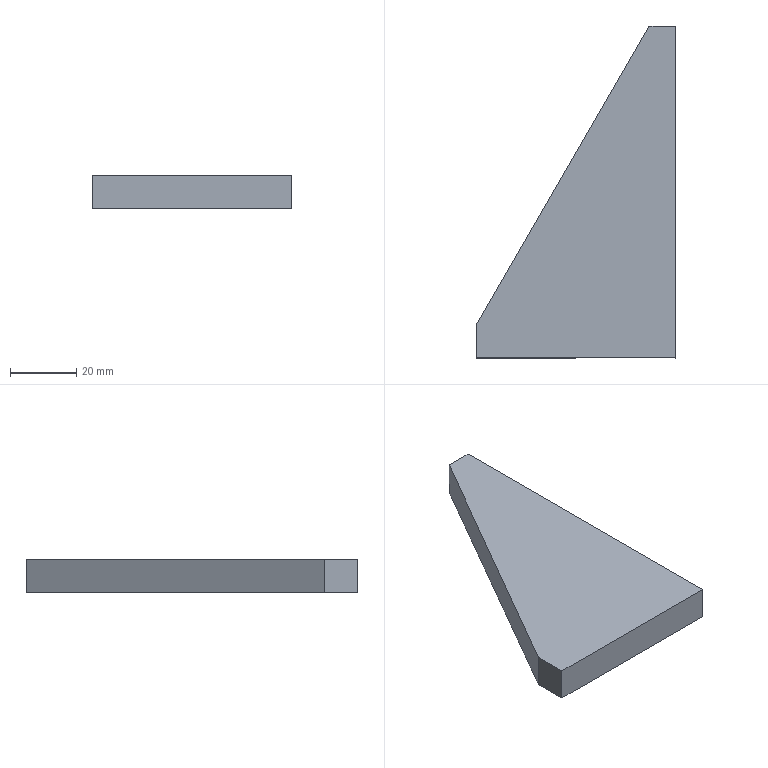Part | STEP file | X77-02104 | 1 solid | 7 faces | box 60 x 100 x 10 mm | volume 36617 mm3 | plane 7
STEP:
#1=CARTESIAN_POINT('',(-109.839,-76.534,0.));
#2=VERTEX_POINT('',#1);
#3=CARTESIAN_POINT('',(-109.839,23.466,0.));
#4=VERTEX_POINT('',#3);
#5=CARTESIAN_POINT('',(-109.839,23.466,0.));
#6=DIRECTION('',(0.,1.,0.));
#7=VECTOR('',#6,1000.);
#8=LINE('',#5,#7);
#9=EDGE_CURVE('',#2,#4,#8,.T.);
#10=ORIENTED_EDGE('',*,*,#9,.T.);
#11=CARTESIAN_POINT('',(-109.839,23.466,10.));
#12=VERTEX_POINT('',#11);
#13=CARTESIAN_POINT('',(-109.839,23.466,10.));
#14=DIRECTION('',(0.,0.,-1.));
#15=VECTOR('',#14,1000.);
#16=LINE('',#13,#15);
#17=EDGE_CURVE('',#12,#4,#16,.T.);
#18=ORIENTED_EDGE('',*,*,#17,.F.);
#19=CARTESIAN_POINT('',(-109.839,-76.534,10.));
#20=VERTEX_POINT('',#19);
#21=CARTESIAN_POINT('',(-109.839,23.466,10.));
#22=DIRECTION('',(0.,1.,0.));
#23=VECTOR('',#22,1000.);
#24=LINE('',#21,#23);
#25=EDGE_CURVE('',#20,#12,#24,.T.);
#26=ORIENTED_EDGE('',*,*,#25,.F.);
#27=CARTESIAN_POINT('',(-109.839,-76.534,10.));
#28=DIRECTION('',(0.,0.,-1.));
#29=VECTOR('',#28,1000.);
#30=LINE('',#27,#29);
#31=EDGE_CURVE('',#20,#2,#30,.T.);
#32=ORIENTED_EDGE('',*,*,#31,.T.);
#33=EDGE_LOOP('',(#10,#18,#26,#32));
#34=FACE_OUTER_BOUND('',#33,.T.);
#35=CARTESIAN_POINT('',(-109.839,23.466,10.));
#36=DIRECTION('',(-1.,0.,0.));
#37=DIRECTION('',(0.,-1.,0.));
#38=AXIS2_PLACEMENT_3D('',#35,#36,#37);
#39=PLANE('',#38);
#40=ADVANCED_FACE('',(#34),#39,.F.);
#41=CARTESIAN_POINT('',(-117.878,23.466,0.));
#42=VERTEX_POINT('',#41);
#43=CARTESIAN_POINT('',(-109.839,23.466,0.));
#44=DIRECTION('',(-1.,0.,0.));
#45=VECTOR('',#44,1000.);
#46=LINE('',#43,#45);
#47=EDGE_CURVE('',#4,#42,#46,.T.);
#48=ORIENTED_EDGE('',*,*,#47,.T.);
#49=CARTESIAN_POINT('',(-117.878,23.466,10.));
#50=VERTEX_POINT('',#49);
#51=CARTESIAN_POINT('',(-117.878,23.466,10.));
#52=DIRECTION('',(0.,0.,-1.));
#53=VECTOR('',#52,1000.);
#54=LINE('',#51,#53);
#55=EDGE_CURVE('',#50,#42,#54,.T.);
#56=ORIENTED_EDGE('',*,*,#55,.F.);
#57=CARTESIAN_POINT('',(-109.839,23.466,10.));
#58=DIRECTION('',(-1.,0.,0.));
#59=VECTOR('',#58,1000.);
#60=LINE('',#57,#59);
#61=EDGE_CURVE('',#12,#50,#60,.T.);
#62=ORIENTED_EDGE('',*,*,#61,.F.);
#63=ORIENTED_EDGE('',*,*,#17,.T.);
#64=EDGE_LOOP('',(#48,#56,#62,#63));
#65=FACE_OUTER_BOUND('',#64,.T.);
#66=CARTESIAN_POINT('',(-109.839,23.466,10.));
#67=DIRECTION('',(0.,-1.,0.));
#68=DIRECTION('',(0.,0.,-1.));
#69=AXIS2_PLACEMENT_3D('',#66,#67,#68);
#70=PLANE('',#69);
#71=ADVANCED_FACE('',(#65),#70,.F.);
#72=CARTESIAN_POINT('',(-169.839,-66.534,0.));
#73=VERTEX_POINT('',#72);
#74=CARTESIAN_POINT('',(-169.839,-66.534,0.));
#75=DIRECTION('',(-0.5,-0.866,0.));
#76=VECTOR('',#75,1000.);
#77=LINE('',#74,#76);
#78=EDGE_CURVE('',#42,#73,#77,.T.);
#79=ORIENTED_EDGE('',*,*,#78,.T.);
#80=CARTESIAN_POINT('',(-169.839,-66.534,10.));
#81=VERTEX_POINT('',#80);
#82=CARTESIAN_POINT('',(-169.839,-66.534,10.));
#83=DIRECTION('',(0.,0.,-1.));
#84=VECTOR('',#83,1000.);
#85=LINE('',#82,#84);
#86=EDGE_CURVE('',#81,#73,#85,.T.);
#87=ORIENTED_EDGE('',*,*,#86,.F.);
#88=CARTESIAN_POINT('',(-169.839,-66.534,10.));
#89=DIRECTION('',(-0.5,-0.866,0.));
#90=VECTOR('',#89,1000.);
#91=LINE('',#88,#90);
#92=EDGE_CURVE('',#50,#81,#91,.T.);
#93=ORIENTED_EDGE('',*,*,#92,.F.);
#94=ORIENTED_EDGE('',*,*,#55,.T.);
#95=EDGE_LOOP('',(#79,#87,#93,#94));
#96=FACE_OUTER_BOUND('',#95,.T.);
#97=CARTESIAN_POINT('',(-169.839,-66.534,10.));
#98=DIRECTION('',(0.866,-0.5,0.));
#99=DIRECTION('',(0.5,0.866,0.));
#100=AXIS2_PLACEMENT_3D('',#97,#98,#99);
#101=PLANE('',#100);
#102=ADVANCED_FACE('',(#96),#101,.F.);
#103=CARTESIAN_POINT('',(-169.839,-76.534,0.));
#104=VERTEX_POINT('',#103);
#105=CARTESIAN_POINT('',(-169.839,-76.534,0.));
#106=DIRECTION('',(0.,-1.,0.));
#107=VECTOR('',#106,1000.);
#108=LINE('',#105,#107);
#109=EDGE_CURVE('',#73,#104,#108,.T.);
#110=ORIENTED_EDGE('',*,*,#109,.T.);
#111=CARTESIAN_POINT('',(-169.839,-76.534,10.));
#112=VERTEX_POINT('',#111);
#113=CARTESIAN_POINT('',(-169.839,-76.534,10.));
#114=DIRECTION('',(0.,0.,-1.));
#115=VECTOR('',#114,1000.);
#116=LINE('',#113,#115);
#117=EDGE_CURVE('',#112,#104,#116,.T.);
#118=ORIENTED_EDGE('',*,*,#117,.F.);
#119=CARTESIAN_POINT('',(-169.839,-76.534,10.));
#120=DIRECTION('',(0.,-1.,0.));
#121=VECTOR('',#120,1000.);
#122=LINE('',#119,#121);
#123=EDGE_CURVE('',#81,#112,#122,.T.);
#124=ORIENTED_EDGE('',*,*,#123,.F.);
#125=ORIENTED_EDGE('',*,*,#86,.T.);
#126=EDGE_LOOP('',(#110,#118,#124,#125));
#127=FACE_OUTER_BOUND('',#126,.T.);
#128=CARTESIAN_POINT('',(-169.839,-76.534,10.));
#129=DIRECTION('',(1.,0.,0.));
#130=DIRECTION('',(0.,0.,-1.));
#131=AXIS2_PLACEMENT_3D('',#128,#129,#130);
#132=PLANE('',#131);
#133=ADVANCED_FACE('',(#127),#132,.F.);
#134=CARTESIAN_POINT('',(-169.839,-76.534,0.));
#135=DIRECTION('',(1.,0.,0.));
#136=VECTOR('',#135,1000.);
#137=LINE('',#134,#136);
#138=EDGE_CURVE('',#104,#2,#137,.T.);
#139=ORIENTED_EDGE('',*,*,#138,.T.);
#140=ORIENTED_EDGE('',*,*,#31,.F.);
#141=CARTESIAN_POINT('',(-169.839,-76.534,10.));
#142=DIRECTION('',(1.,0.,0.));
#143=VECTOR('',#142,1000.);
#144=LINE('',#141,#143);
#145=EDGE_CURVE('',#112,#20,#144,.T.);
#146=ORIENTED_EDGE('',*,*,#145,.F.);
#147=ORIENTED_EDGE('',*,*,#117,.T.);
#148=EDGE_LOOP('',(#139,#140,#146,#147));
#149=FACE_OUTER_BOUND('',#148,.T.);
#150=CARTESIAN_POINT('',(-169.839,-76.534,10.));
#151=DIRECTION('',(0.,1.,0.));
#152=DIRECTION('',(-1.,0.,0.));
#153=AXIS2_PLACEMENT_3D('',#150,#151,#152);
#154=PLANE('',#153);
#155=ADVANCED_FACE('',(#149),#154,.F.);
#156=ORIENTED_EDGE('',*,*,#25,.T.);
#157=ORIENTED_EDGE('',*,*,#61,.T.);
#158=ORIENTED_EDGE('',*,*,#92,.T.);
#159=ORIENTED_EDGE('',*,*,#123,.T.);
#160=ORIENTED_EDGE('',*,*,#145,.T.);
#161=EDGE_LOOP('',(#156,#157,#158,#159,#160));
#162=FACE_OUTER_BOUND('',#161,.T.);
#163=CARTESIAN_POINT('',(-109.839,-76.534,10.));
#164=DIRECTION('',(0.,0.,1.));
#165=DIRECTION('',(1.,0.,0.));
#166=AXIS2_PLACEMENT_3D('',#163,#164,#165);
#167=PLANE('',#166);
#168=ADVANCED_FACE('',(#162),#167,.T.);
#169=ORIENTED_EDGE('',*,*,#9,.F.);
#170=ORIENTED_EDGE('',*,*,#138,.F.);
#171=ORIENTED_EDGE('',*,*,#109,.F.);
#172=ORIENTED_EDGE('',*,*,#78,.F.);
#173=ORIENTED_EDGE('',*,*,#47,.F.);
#174=EDGE_LOOP('',(#169,#170,#171,#172,#173));
#175=FACE_OUTER_BOUND('',#174,.T.);
#176=CARTESIAN_POINT('',(-109.839,-76.534,0.));
#177=DIRECTION('',(0.,0.,1.));
#178=DIRECTION('',(1.,0.,0.));
#179=AXIS2_PLACEMENT_3D('',#176,#177,#178);
#180=PLANE('',#179);
#181=ADVANCED_FACE('',(#175),#180,.F.);
#182=CLOSED_SHELL('',(#40,#71,#102,#133,#155,#168,#181));
#183=MANIFOLD_SOLID_BREP('',#182);
#184=CARTESIAN_POINT('',(0.,0.,0.));
#185=DIRECTION('',(0.,0.,1.));
#186=DIRECTION('',(1.,0.,0.));
#187=AXIS2_PLACEMENT_3D('',#184,#185,#186);
#188=(LENGTH_UNIT()NAMED_UNIT(*)SI_UNIT(.MILLI.,.METRE.));
#189=UNCERTAINTY_MEASURE_WITH_UNIT(LENGTH_MEASURE(0.00001),#188,'','');
#190=(NAMED_UNIT(*)PLANE_ANGLE_UNIT()SI_UNIT($,.RADIAN.));
#191=(NAMED_UNIT(*)SI_UNIT($,.STERADIAN.)SOLID_ANGLE_UNIT());
#192=(GEOMETRIC_REPRESENTATION_CONTEXT(3)GLOBAL_UNCERTAINTY_ASSIGNED_CONTEXT((#189))GLOBAL_UNIT_ASSIGNED_CONTEXT((#188,#190,#191))REPRESENTATION_CONTEXT('',''));
#193=ADVANCED_BREP_SHAPE_REPRESENTATION('',(#183,#187),#192);